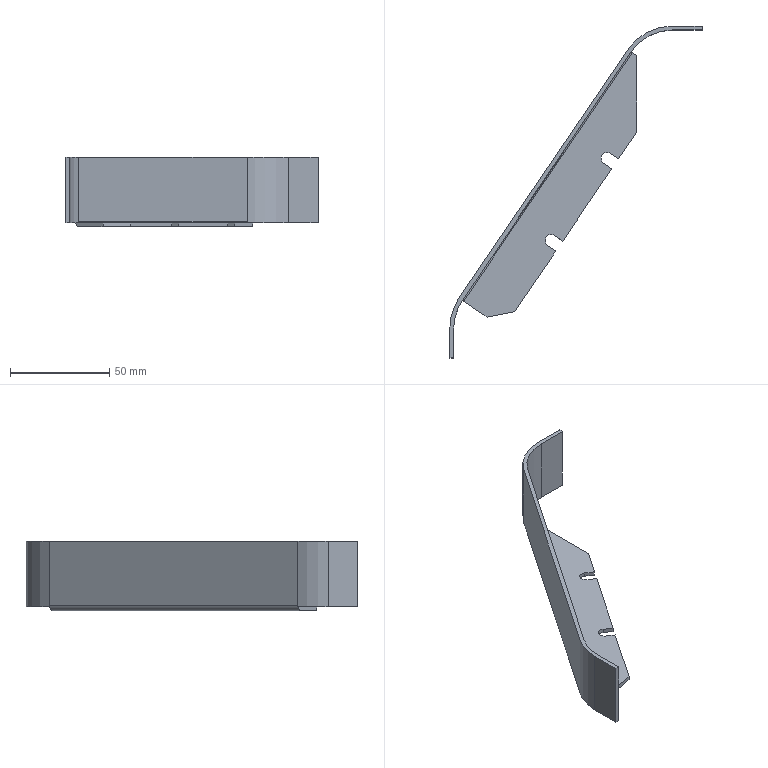Part | STEP file | 10020103U05P16_default | 1 solid | 34 faces | box 127 x 167 x 35 mm | volume 21616 mm3 | plane 26 | cylinder 8 | commonest cylinder face diameters 6 x2 50 x2 54 x2 1.473 x1 5.473 x1